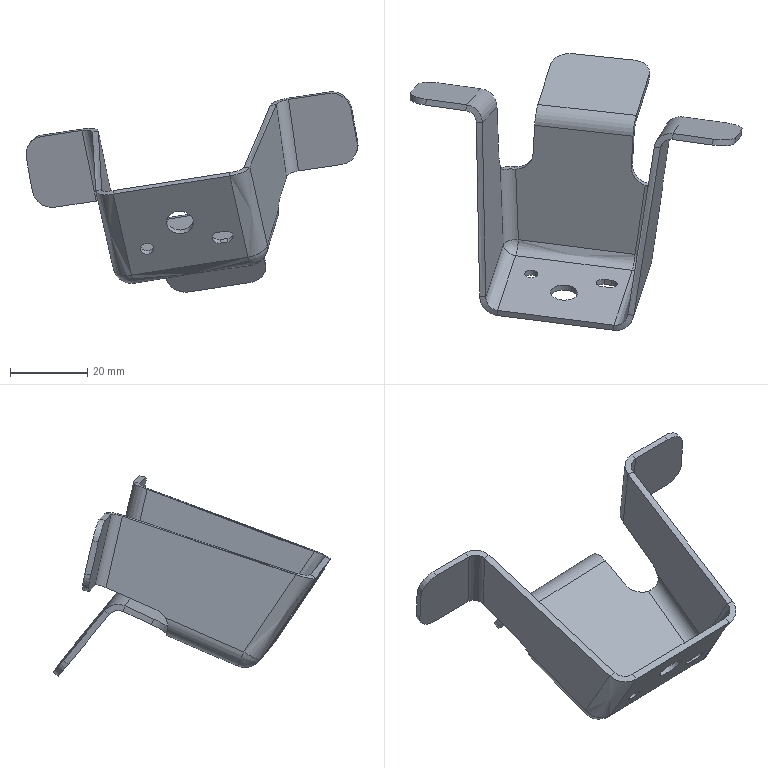Part | STEP file | FNA5401391 | 1 solid | 82 faces | box 86.183 x 71.891 x 52.032 mm | volume 9472 mm3 | spline 55 | cylinder 12 | plane 9 | sphere 4 | other 2 | commonest cylinder face diameters 10 x4 6 x3 9.2 x3 6.8 x2